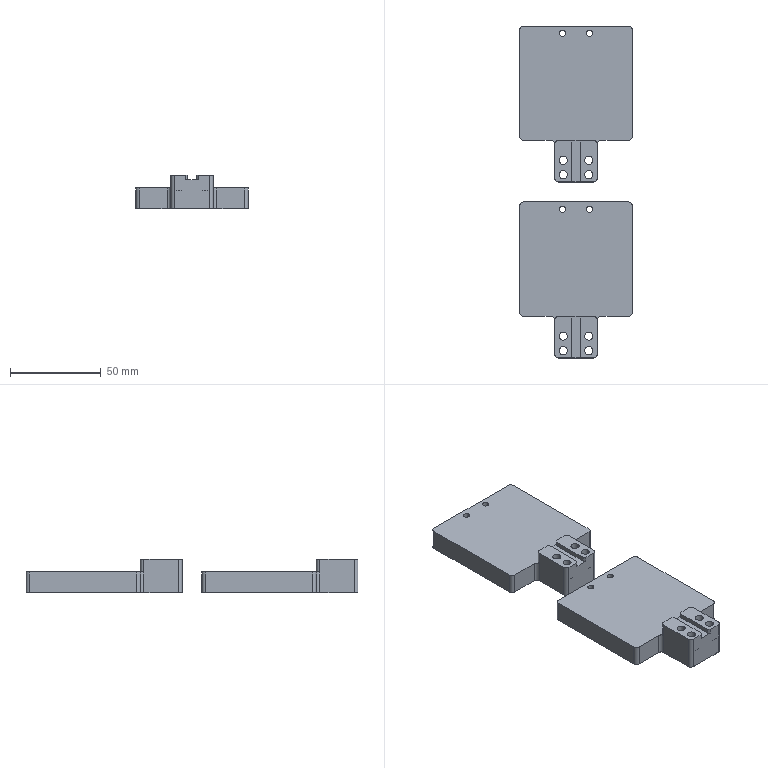NC program | NX | posted with a generic post | part box 62 x 183 x 18.5 mm
Lines 4184 to 4383 of 4383:
(PLANAR_MILL_COPY , TOOL : D6A45)
N8324 T01 M6
N8326 G54
N8328 G17 G0 G90 X3.5 Y38.933 S9500 M3
N8330 G43 Z30. H1
N8332 Z0.5
N8334 G94 G1 Z-1. F1250.
N8336 G3 X3.25 Y38.5 R0.5
N8338 X4. Y37.75 R0.75
N8340 X3.25 Y38.5 R-0.75
N8342 X3.5 Y38.067 R0.5
N8344 G1 Z0.5
N8346 G0 Z30.
N8348 Y23.933
N8350 Z0.5
N8352 G1 Z-1.
N8354 G3 X3.25 Y23.5 R0.5
N8356 X4. Y22.75 R0.75
N8358 X3.25 Y23.5 R-0.75
N8360 X3.5 Y23.067 R0.5
N8362 G1 Z0.5
N8364 G0 Z30.
N8366 X-1.4 Y30.134
N8368 Z0.5
N8370 G1 Z-1.
N8372 G3 X-0.9 Y31. R1.
N8374 G1 Y60.
N8376 G2 X2. Y62.9 R2.9
N8378 G1 X61.
N8380 G2 X63.9 Y60. R2.9
N8382 G1 Y44.7
N8384 G3 X65. Y43.6 R1.1
N8386 G1 X84.
N8388 G2 X86.9 Y40.7 R2.9
N8390 G1 Y21.3
N8392 G2 X84. Y18.4 R2.9
N8394 G1 X65.
N8396 G3 X63.9 Y17.3 R1.1
N8398 G1 Y2.
N8400 G2 X61. Y-0.9 R2.9
N8402 G1 X2.
N8404 G2 X-0.9 Y2. R2.9
N8406 G1 Y31.
N8408 G3 X-1.4 Y31.866 R1.
N8410 G1 Z0.5
N8412 G0 Z30.
N8414 X65.567 Y23.
N8416 Z0.5
N8418 G1 Z-1.
N8420 G3 X66. Y22.75 R0.5
N8422 X66.75 Y23.5 R0.75
N8424 X66. Y22.75 R-0.75
N8426 X66.433 Y23. R0.5
N8428 G1 Z0.5
N8430 G0 Z30.
N8432 X73.134 Y21.35
N8434 Z0.5
N8436 G1 Z-1.
N8438 G3 X74. Y20.85 R1.
N8440 X77.05 Y23.9 R3.05
N8442 X74. Y20.85 R-3.05
N8444 X74.866 Y21.35 R1.
N8446 G1 Z0.5
N8448 G0 Z30.
N8450 X66.433 Y39.
N8452 Z0.5
N8454 G1 Z-1.
N8456 G3 X66. Y39.25 R0.5
N8458 X65.25 Y38.5 R0.75
N8460 X66. Y39.25 R-0.75
N8462 X65.567 Y39. R0.5
N8464 G1 Z0.5
N8466 G0 Z30.
N8468 X74.866 Y40.65
N8470 Z0.5
N8472 G1 Z-1.
N8474 G3 X74. Y41.15 R1.
N8476 X70.95 Y38.1 R3.05
N8478 X74. Y41.15 R-3.05
N8480 X73.134 Y40.65 R1.
N8482 G1 Z0.5
N8484 G0 Z30.
N8486 X82.866
N8488 Z0.5
N8490 G1 Z-1.
N8492 G3 X82. Y41.15 R1.
N8494 X78.95 Y38.1 R3.05
N8496 X82. Y41.15 R-3.05
N8498 X81.134 Y40.65 R1.
N8500 G1 Z0.5
N8502 G0 Z30.
N8504 Y21.35
N8506 Z0.5
N8508 G1 Z-1.
N8510 G3 X82. Y20.85 R1.
N8512 X85.05 Y23.9 R3.05
N8514 X82. Y20.85 R-3.05
N8516 X82.866 Y21.35 R1.
N8518 G1 Z0.5
N8520 G0 Z30.
N8522 X100.567 Y23.
N8524 Z0.5
N8526 G1 Z-1.
N8528 G3 X101. Y22.75 R0.5
N8530 X101.75 Y23.5 R0.75
N8532 X101. Y22.75 R-0.75
N8534 X101.433 Y23. R0.5
N8536 G1 Z0.5
N8538 G0 Z30.
N8540 Y39.
N8542 Z0.5
N8544 G1 Z-1.
N8546 G3 X101. Y39.25 R0.5
N8548 X100.25 Y38.5 R0.75
N8550 X101. Y39.25 R-0.75
N8552 X100.567 Y39. R0.5
N8554 G1 Z0.5
N8556 G0 Z30.
N8558 X127.634 Y63.4
N8560 Z0.5
N8562 G1 Z-1.
N8564 G3 X128.5 Y62.9 R1.
N8566 G1 X158.
N8568 G2 X160.9 Y60. R2.9
N8570 G1 Y44.7
N8572 G3 X162. Y43.6 R1.1
N8574 G1 X181.
N8576 G2 X183.9 Y40.7 R2.9
N8578 G1 Y21.3
N8580 G2 X181. Y18.4 R2.9
N8582 G1 X162.
N8584 G3 X160.9 Y17.3 R1.1
N8586 G1 Y2.
N8588 G2 X158. Y-0.9 R2.9
N8590 G1 X99.
N8592 G2 X96.1 Y2. R2.9
N8594 G1 Y60.
N8596 G2 X99. Y62.9 R2.9
N8598 G1 X128.5
N8600 G3 X129.366 Y63.4 R1.
N8602 G1 Z0.5
N8604 G0 Z30.
N8606 X163.5 Y23.067
N8608 Z0.5
N8610 G1 Z-1.
N8612 G3 X163.75 Y23.5 R0.5
N8614 X163. Y24.25 R0.75
N8616 X163.75 Y23.5 R-0.75
N8618 X163.5 Y23.933 R0.5
N8620 G1 Z0.5
N8622 G0 Z30.
N8624 X173.55 Y23.034
N8626 Z0.5
N8628 G1 Z-1.
N8630 G3 X174.05 Y23.9 R1.
N8632 X171. Y26.95 R3.05
N8634 X174.05 Y23.9 R-3.05
N8636 X173.55 Y24.766 R1.
N8638 G1 Z0.5
N8640 G0 Z30.
N8642 X181.55 Y23.034
N8644 Z0.5
N8646 G1 Z-1.
N8648 G3 X182.05 Y23.9 R1.
N8650 X179. Y26.95 R3.05
N8652 X182.05 Y23.9 R-3.05
N8654 X181.55 Y24.766 R1.
N8656 G1 Z0.5
N8658 G0 Z30.
N8660 Y37.234
N8662 Z0.5
N8664 G1 Z-1.
N8666 G3 X182.05 Y38.1 R1.
N8668 X179. Y41.15 R3.05
N8670 X182.05 Y38.1 R-3.05
N8672 X181.55 Y38.966 R1.
N8674 G1 Z0.5
N8676 G0 Z30.
N8678 X173.55 Y37.234
N8680 Z0.5
N8682 G1 Z-1.
N8684 G3 X174.05 Y38.1 R1.
N8686 X171. Y41.15 R3.05
N8688 X174.05 Y38.1 R-3.05
N8690 X173.55 Y38.966 R1.
N8692 G1 Z0.5
N8694 G0 Z30.
N8696 X163.5 Y38.067
N8698 Z0.5
N8700 G1 Z-1.
N8702 G3 X163.75 Y38.5 R0.5
N8704 X163. Y39.25 R0.75
N8706 X163.75 Y38.5 R-0.75
N8708 X163.5 Y38.933 R0.5
N8710 G1 Z0.5
N8712 G0 Z30.
N8714 M5
N8716 M2